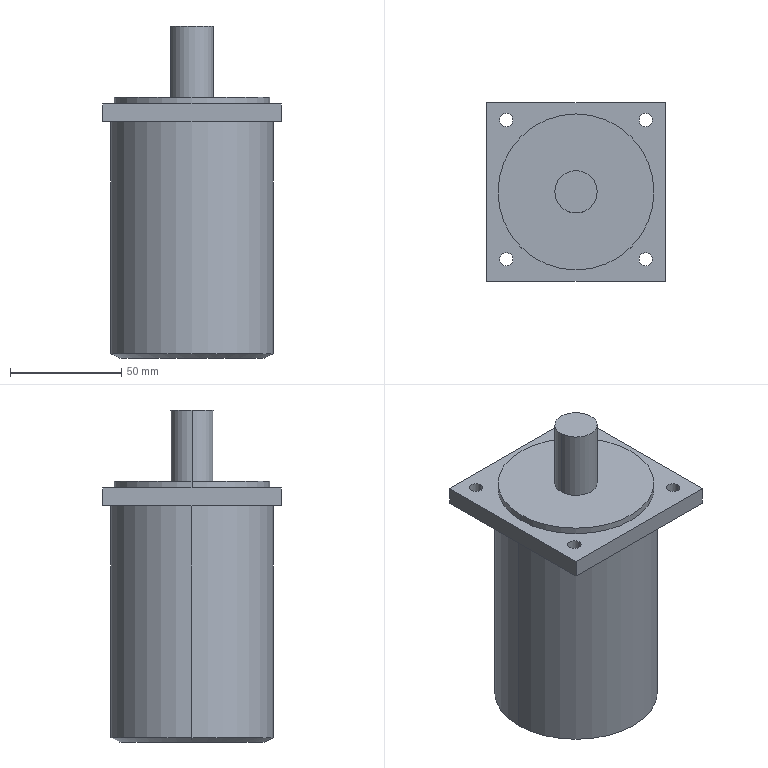Part | SolidWorks | features Boss 3, Chamfer 1, Cut 1, Extrusion 1 | 1 solid | 25 faces | box 80 x 80 x 149 mm | volume 513498 mm3 | cylinder 14 | plane 9 | cone 2 | commonest cylinder face diameters 6 x8 19 x2 70 x2 72.985 x2
STEP:
#1=CARTESIAN_POINT('',(7.508,40.,-106.));
#2=VERTEX_POINT('',#1);
#3=CARTESIAN_POINT('',(72.492,40.,-106.));
#4=VERTEX_POINT('',#3);
#5=CARTESIAN_POINT('',(40.,40.,-106.));
#6=DIRECTION('',(0.,0.,-1.));
#7=DIRECTION('',(-1.,0.,0.));
#8=AXIS2_PLACEMENT_3D('',#5,#6,#7);
#9=CIRCLE('',#8,32.492);
#10=EDGE_CURVE('',#2,#4,#9,.T.);
#11=ORIENTED_EDGE('',*,*,#10,.F.);
#12=CARTESIAN_POINT('',(3.508,40.,-104.));
#13=VERTEX_POINT('',#12);
#14=CARTESIAN_POINT('',(7.508,40.,-106.));
#15=DIRECTION('',(-0.8944,0.,0.4472));
#16=VECTOR('',#15,1000.);
#17=LINE('',#14,#16);
#18=EDGE_CURVE('',#2,#13,#17,.T.);
#19=ORIENTED_EDGE('',*,*,#18,.T.);
#20=CARTESIAN_POINT('',(76.492,40.,-104.));
#21=VERTEX_POINT('',#20);
#22=CARTESIAN_POINT('',(40.,40.,-104.));
#23=DIRECTION('',(0.,0.,1.));
#24=DIRECTION('',(-1.,0.,0.));
#25=AXIS2_PLACEMENT_3D('',#22,#23,#24);
#26=CIRCLE('',#25,36.492);
#27=EDGE_CURVE('',#21,#13,#26,.T.);
#28=ORIENTED_EDGE('',*,*,#27,.F.);
#29=CARTESIAN_POINT('',(72.492,40.,-106.));
#30=DIRECTION('',(0.8944,0.,0.4472));
#31=VECTOR('',#30,1000.);
#32=LINE('',#29,#31);
#33=EDGE_CURVE('',#4,#21,#32,.T.);
#34=ORIENTED_EDGE('',*,*,#33,.F.);
#35=EDGE_LOOP('',(#11,#19,#28,#34));
#36=FACE_OUTER_BOUND('',#35,.T.);
#37=CARTESIAN_POINT('',(40.,40.,-106.));
#38=DIRECTION('',(0.,0.,1.));
#39=DIRECTION('',(1.,0.,0.));
#40=AXIS2_PLACEMENT_3D('',#37,#38,#39);
#41=CONICAL_SURFACE('',#40,32.492,1.107);
#42=ADVANCED_FACE('',(#36),#41,.T.);
#43=CARTESIAN_POINT('',(5.714,9.772,0.));
#44=VERTEX_POINT('',#43);
#45=CARTESIAN_POINT('',(11.714,9.772,0.));
#46=VERTEX_POINT('',#45);
#47=CARTESIAN_POINT('',(8.714,9.772,0.));
#48=DIRECTION('',(0.,0.,1.));
#49=DIRECTION('',(-1.,0.,0.));
#50=AXIS2_PLACEMENT_3D('',#47,#48,#49);
#51=CIRCLE('',#50,3.);
#52=EDGE_CURVE('',#44,#46,#51,.T.);
#53=ORIENTED_EDGE('',*,*,#52,.F.);
#54=CARTESIAN_POINT('',(5.714,9.772,8.));
#55=VERTEX_POINT('',#54);
#56=CARTESIAN_POINT('',(5.714,9.772,-106.001));
#57=DIRECTION('',(0.,0.,1.));
#58=VECTOR('',#57,1000.);
#59=LINE('',#56,#58);
#60=EDGE_CURVE('',#44,#55,#59,.T.);
#61=ORIENTED_EDGE('',*,*,#60,.T.);
#62=CARTESIAN_POINT('',(11.714,9.772,8.));
#63=VERTEX_POINT('',#62);
#64=CARTESIAN_POINT('',(8.714,9.772,8.));
#65=DIRECTION('',(0.,0.,1.));
#66=DIRECTION('',(1.,0.,0.));
#67=AXIS2_PLACEMENT_3D('',#64,#65,#66);
#68=CIRCLE('',#67,3.);
#69=EDGE_CURVE('',#55,#63,#68,.T.);
#70=ORIENTED_EDGE('',*,*,#69,.T.);
#71=CARTESIAN_POINT('',(11.714,9.772,-106.001));
#72=DIRECTION('',(0.,0.,1.));
#73=VECTOR('',#72,1000.);
#74=LINE('',#71,#73);
#75=EDGE_CURVE('',#46,#63,#74,.T.);
#76=ORIENTED_EDGE('',*,*,#75,.F.);
#77=EDGE_LOOP('',(#53,#61,#70,#76));
#78=FACE_OUTER_BOUND('',#77,.T.);
#79=CARTESIAN_POINT('',(8.714,9.772,-106.001));
#80=DIRECTION('',(0.,0.,1.));
#81=DIRECTION('',(1.,0.,0.));
#82=AXIS2_PLACEMENT_3D('',#79,#80,#81);
#83=CYLINDRICAL_SURFACE('',#82,3.);
#84=ADVANCED_FACE('',(#78),#83,.F.);
#85=CARTESIAN_POINT('',(68.286,9.772,0.));
#86=VERTEX_POINT('',#85);
#87=CARTESIAN_POINT('',(74.286,9.772,0.));
#88=VERTEX_POINT('',#87);
#89=CARTESIAN_POINT('',(71.286,9.772,0.));
#90=DIRECTION('',(0.,0.,1.));
#91=DIRECTION('',(-1.,0.,0.));
#92=AXIS2_PLACEMENT_3D('',#89,#90,#91);
#93=CIRCLE('',#92,3.);
#94=EDGE_CURVE('',#86,#88,#93,.T.);
#95=ORIENTED_EDGE('',*,*,#94,.F.);
#96=CARTESIAN_POINT('',(68.286,9.772,8.));
#97=VERTEX_POINT('',#96);
#98=CARTESIAN_POINT('',(68.286,9.772,-106.001));
#99=DIRECTION('',(0.,0.,1.));
#100=VECTOR('',#99,1000.);
#101=LINE('',#98,#100);
#102=EDGE_CURVE('',#86,#97,#101,.T.);
#103=ORIENTED_EDGE('',*,*,#102,.T.);
#104=CARTESIAN_POINT('',(74.286,9.772,8.));
#105=VERTEX_POINT('',#104);
#106=CARTESIAN_POINT('',(71.286,9.772,8.));
#107=DIRECTION('',(0.,0.,1.));
#108=DIRECTION('',(1.,0.,0.));
#109=AXIS2_PLACEMENT_3D('',#106,#107,#108);
#110=CIRCLE('',#109,3.);
#111=EDGE_CURVE('',#97,#105,#110,.T.);
#112=ORIENTED_EDGE('',*,*,#111,.T.);
#113=CARTESIAN_POINT('',(74.286,9.772,-106.001));
#114=DIRECTION('',(0.,0.,1.));
#115=VECTOR('',#114,1000.);
#116=LINE('',#113,#115);
#117=EDGE_CURVE('',#88,#105,#116,.T.);
#118=ORIENTED_EDGE('',*,*,#117,.F.);
#119=EDGE_LOOP('',(#95,#103,#112,#118));
#120=FACE_OUTER_BOUND('',#119,.T.);
#121=CARTESIAN_POINT('',(71.286,9.772,-106.001));
#122=DIRECTION('',(0.,0.,1.));
#123=DIRECTION('',(1.,0.,0.));
#124=AXIS2_PLACEMENT_3D('',#121,#122,#123);
#125=CYLINDRICAL_SURFACE('',#124,3.);
#126=ADVANCED_FACE('',(#120),#125,.F.);
#127=CARTESIAN_POINT('',(68.286,72.344,0.));
#128=VERTEX_POINT('',#127);
#129=CARTESIAN_POINT('',(74.286,72.344,0.));
#130=VERTEX_POINT('',#129);
#131=CARTESIAN_POINT('',(71.286,72.344,0.));
#132=DIRECTION('',(0.,0.,1.));
#133=DIRECTION('',(-1.,0.,0.));
#134=AXIS2_PLACEMENT_3D('',#131,#132,#133);
#135=CIRCLE('',#134,3.);
#136=EDGE_CURVE('',#128,#130,#135,.T.);
#137=ORIENTED_EDGE('',*,*,#136,.F.);
#138=CARTESIAN_POINT('',(68.286,72.344,8.));
#139=VERTEX_POINT('',#138);
#140=CARTESIAN_POINT('',(68.286,72.344,-106.001));
#141=DIRECTION('',(0.,0.,1.));
#142=VECTOR('',#141,1000.);
#143=LINE('',#140,#142);
#144=EDGE_CURVE('',#128,#139,#143,.T.);
#145=ORIENTED_EDGE('',*,*,#144,.T.);
#146=CARTESIAN_POINT('',(74.286,72.344,8.));
#147=VERTEX_POINT('',#146);
#148=CARTESIAN_POINT('',(71.286,72.344,8.));
#149=DIRECTION('',(0.,0.,1.));
#150=DIRECTION('',(1.,0.,0.));
#151=AXIS2_PLACEMENT_3D('',#148,#149,#150);
#152=CIRCLE('',#151,3.);
#153=EDGE_CURVE('',#139,#147,#152,.T.);
#154=ORIENTED_EDGE('',*,*,#153,.T.);
#155=CARTESIAN_POINT('',(74.286,72.344,-106.001));
#156=DIRECTION('',(0.,0.,1.));
#157=VECTOR('',#156,1000.);
#158=LINE('',#155,#157);
#159=EDGE_CURVE('',#130,#147,#158,.T.);
#160=ORIENTED_EDGE('',*,*,#159,.F.);
#161=EDGE_LOOP('',(#137,#145,#154,#160));
#162=FACE_OUTER_BOUND('',#161,.T.);
#163=CARTESIAN_POINT('',(71.286,72.344,-106.001));
#164=DIRECTION('',(0.,0.,1.));
#165=DIRECTION('',(1.,0.,0.));
#166=AXIS2_PLACEMENT_3D('',#163,#164,#165);
#167=CYLINDRICAL_SURFACE('',#166,3.);
#168=ADVANCED_FACE('',(#162),#167,.F.);
#169=CARTESIAN_POINT('',(5.714,72.344,0.));
#170=VERTEX_POINT('',#169);
#171=CARTESIAN_POINT('',(11.714,72.344,0.));
#172=VERTEX_POINT('',#171);
#173=CARTESIAN_POINT('',(8.714,72.344,0.));
#174=DIRECTION('',(0.,0.,1.));
#175=DIRECTION('',(-1.,0.,0.));
#176=AXIS2_PLACEMENT_3D('',#173,#174,#175);
#177=CIRCLE('',#176,3.);
#178=EDGE_CURVE('',#170,#172,#177,.T.);
#179=ORIENTED_EDGE('',*,*,#178,.F.);
#180=CARTESIAN_POINT('',(5.714,72.344,8.));
#181=VERTEX_POINT('',#180);
#182=CARTESIAN_POINT('',(5.714,72.344,-106.001));
#183=DIRECTION('',(0.,0.,1.));
#184=VECTOR('',#183,1000.);
#185=LINE('',#182,#184);
#186=EDGE_CURVE('',#170,#181,#185,.T.);
#187=ORIENTED_EDGE('',*,*,#186,.T.);
#188=CARTESIAN_POINT('',(11.714,72.344,8.));
#189=VERTEX_POINT('',#188);
#190=CARTESIAN_POINT('',(8.714,72.344,8.));
#191=DIRECTION('',(0.,0.,1.));
#192=DIRECTION('',(1.,0.,0.));
#193=AXIS2_PLACEMENT_3D('',#190,#191,#192);
#194=CIRCLE('',#193,3.);
#195=EDGE_CURVE('',#181,#189,#194,.T.);
#196=ORIENTED_EDGE('',*,*,#195,.T.);
#197=CARTESIAN_POINT('',(11.714,72.344,-106.001));
#198=DIRECTION('',(0.,0.,1.));
#199=VECTOR('',#198,1000.);
#200=LINE('',#197,#199);
#201=EDGE_CURVE('',#172,#189,#200,.T.);
#202=ORIENTED_EDGE('',*,*,#201,.F.);
#203=EDGE_LOOP('',(#179,#187,#196,#202));
#204=FACE_OUTER_BOUND('',#203,.T.);
#205=CARTESIAN_POINT('',(8.714,72.344,-106.001));
#206=DIRECTION('',(0.,0.,1.));
#207=DIRECTION('',(1.,0.,0.));
#208=AXIS2_PLACEMENT_3D('',#205,#206,#207);
#209=CYLINDRICAL_SURFACE('',#208,3.);
#210=ADVANCED_FACE('',(#204),#209,.F.);
#211=ORIENTED_EDGE('',*,*,#27,.T.);
#212=CARTESIAN_POINT('',(3.508,40.,0.));
#213=VERTEX_POINT('',#212);
#214=CARTESIAN_POINT('',(3.508,40.,-106.));
#215=DIRECTION('',(0.,0.,1.));
#216=VECTOR('',#215,1000.);
#217=LINE('',#214,#216);
#218=EDGE_CURVE('',#13,#213,#217,.T.);
#219=ORIENTED_EDGE('',*,*,#218,.T.);
#220=CARTESIAN_POINT('',(76.492,40.,0.));
#221=VERTEX_POINT('',#220);
#222=CARTESIAN_POINT('',(40.,40.,0.));
#223=DIRECTION('',(0.,0.,-1.));
#224=DIRECTION('',(-1.,0.,0.));
#225=AXIS2_PLACEMENT_3D('',#222,#223,#224);
#226=CIRCLE('',#225,36.492);
#227=EDGE_CURVE('',#213,#221,#226,.T.);
#228=ORIENTED_EDGE('',*,*,#227,.T.);
#229=CARTESIAN_POINT('',(76.492,40.,-106.));
#230=DIRECTION('',(0.,0.,1.));
#231=VECTOR('',#230,1000.);
#232=LINE('',#229,#231);
#233=EDGE_CURVE('',#21,#221,#232,.T.);
#234=ORIENTED_EDGE('',*,*,#233,.F.);
#235=EDGE_LOOP('',(#211,#219,#228,#234));
#236=FACE_OUTER_BOUND('',#235,.T.);
#237=CARTESIAN_POINT('',(40.,40.,-106.));
#238=DIRECTION('',(0.,0.,1.));
#239=DIRECTION('',(1.,0.,0.));
#240=AXIS2_PLACEMENT_3D('',#237,#238,#239);
#241=CYLINDRICAL_SURFACE('',#240,36.492);
#242=ADVANCED_FACE('',(#236),#241,.T.);
#243=CARTESIAN_POINT('',(49.5,40.,43.));
#244=VERTEX_POINT('',#243);
#245=CARTESIAN_POINT('',(30.5,40.,43.));
#246=VERTEX_POINT('',#245);
#247=CARTESIAN_POINT('',(40.,40.,43.));
#248=DIRECTION('',(0.,0.,1.));
#249=DIRECTION('',(1.,0.,0.));
#250=AXIS2_PLACEMENT_3D('',#247,#248,#249);
#251=CIRCLE('',#250,9.5);
#252=EDGE_CURVE('',#244,#246,#251,.T.);
#253=ORIENTED_EDGE('',*,*,#252,.F.);
#254=CARTESIAN_POINT('',(49.5,40.,11.));
#255=VERTEX_POINT('',#254);
#256=CARTESIAN_POINT('',(49.5,40.,43.));
#257=DIRECTION('',(0.,0.,-1.));
#258=VECTOR('',#257,1000.);
#259=LINE('',#256,#258);
#260=EDGE_CURVE('',#244,#255,#259,.T.);
#261=ORIENTED_EDGE('',*,*,#260,.T.);
#262=CARTESIAN_POINT('',(30.5,40.,11.));
#263=VERTEX_POINT('',#262);
#264=CARTESIAN_POINT('',(40.,40.,11.));
#265=DIRECTION('',(0.,0.,1.));
#266=DIRECTION('',(1.,0.,0.));
#267=AXIS2_PLACEMENT_3D('',#264,#265,#266);
#268=CIRCLE('',#267,9.5);
#269=EDGE_CURVE('',#255,#263,#268,.T.);
#270=ORIENTED_EDGE('',*,*,#269,.T.);
#271=CARTESIAN_POINT('',(30.5,40.,43.));
#272=DIRECTION('',(0.,0.,-1.));
#273=VECTOR('',#272,1000.);
#274=LINE('',#271,#273);
#275=EDGE_CURVE('',#246,#263,#274,.T.);
#276=ORIENTED_EDGE('',*,*,#275,.F.);
#277=EDGE_LOOP('',(#253,#261,#270,#276));
#278=FACE_OUTER_BOUND('',#277,.T.);
#279=CARTESIAN_POINT('',(40.,40.,43.));
#280=DIRECTION('',(0.,0.,-1.));
#281=DIRECTION('',(-1.,0.,0.));
#282=AXIS2_PLACEMENT_3D('',#279,#280,#281);
#283=CYLINDRICAL_SURFACE('',#282,9.5);
#284=ADVANCED_FACE('',(#278),#283,.T.);
#285=CARTESIAN_POINT('',(75.,40.,11.));
#286=VERTEX_POINT('',#285);
#287=CARTESIAN_POINT('',(5.,40.,11.));
#288=VERTEX_POINT('',#287);
#289=CARTESIAN_POINT('',(40.,40.,11.));
#290=DIRECTION('',(0.,0.,1.));
#291=DIRECTION('',(1.,0.,0.));
#292=AXIS2_PLACEMENT_3D('',#289,#290,#291);
#293=CIRCLE('',#292,35.);
#294=EDGE_CURVE('',#286,#288,#293,.T.);
#295=ORIENTED_EDGE('',*,*,#294,.F.);
#296=CARTESIAN_POINT('',(75.,40.,8.));
#297=VERTEX_POINT('',#296);
#298=CARTESIAN_POINT('',(75.,40.,11.));
#299=DIRECTION('',(0.,0.,-1.));
#300=VECTOR('',#299,1000.);
#301=LINE('',#298,#300);
#302=EDGE_CURVE('',#286,#297,#301,.T.);
#303=ORIENTED_EDGE('',*,*,#302,.T.);
#304=CARTESIAN_POINT('',(5.,40.,8.));
#305=VERTEX_POINT('',#304);
#306=CARTESIAN_POINT('',(40.,40.,8.));
#307=DIRECTION('',(0.,0.,1.));
#308=DIRECTION('',(-1.,0.,0.));
#309=AXIS2_PLACEMENT_3D('',#306,#307,#308);
#310=CIRCLE('',#309,35.);
#311=EDGE_CURVE('',#297,#305,#310,.T.);
#312=ORIENTED_EDGE('',*,*,#311,.T.);
#313=CARTESIAN_POINT('',(5.,40.,11.));
#314=DIRECTION('',(0.,0.,-1.));
#315=VECTOR('',#314,1000.);
#316=LINE('',#313,#315);
#317=EDGE_CURVE('',#288,#305,#316,.T.);
#318=ORIENTED_EDGE('',*,*,#317,.F.);
#319=EDGE_LOOP('',(#295,#303,#312,#318));
#320=FACE_OUTER_BOUND('',#319,.T.);
#321=CARTESIAN_POINT('',(40.,40.,11.));
#322=DIRECTION('',(0.,0.,-1.));
#323=DIRECTION('',(-1.,0.,0.));
#324=AXIS2_PLACEMENT_3D('',#321,#322,#323);
#325=CYLINDRICAL_SURFACE('',#324,35.);
#326=ADVANCED_FACE('',(#320),#325,.T.);
#327=CARTESIAN_POINT('',(8.714,9.772,0.));
#328=DIRECTION('',(0.,0.,1.));
#329=DIRECTION('',(-1.,0.,0.));
#330=AXIS2_PLACEMENT_3D('',#327,#328,#329);
#331=CIRCLE('',#330,3.);
#332=EDGE_CURVE('',#46,#44,#331,.T.);
#333=ORIENTED_EDGE('',*,*,#332,.T.);
#334=ORIENTED_EDGE('',*,*,#52,.T.);
#335=EDGE_LOOP('',(#333,#334));
#336=FACE_BOUND('',#335,.T.);
#337=CARTESIAN_POINT('',(71.286,9.772,0.));
#338=DIRECTION('',(0.,0.,1.));
#339=DIRECTION('',(-1.,0.,0.));
#340=AXIS2_PLACEMENT_3D('',#337,#338,#339);
#341=CIRCLE('',#340,3.);
#342=EDGE_CURVE('',#88,#86,#341,.T.);
#343=ORIENTED_EDGE('',*,*,#342,.T.);
#344=ORIENTED_EDGE('',*,*,#94,.T.);
#345=EDGE_LOOP('',(#343,#344));
#346=FACE_BOUND('',#345,.T.);
#347=CARTESIAN_POINT('',(71.286,72.344,0.));
#348=DIRECTION('',(0.,0.,1.));
#349=DIRECTION('',(-1.,0.,0.));
#350=AXIS2_PLACEMENT_3D('',#347,#348,#349);
#351=CIRCLE('',#350,3.);
#352=EDGE_CURVE('',#130,#128,#351,.T.);
#353=ORIENTED_EDGE('',*,*,#352,.T.);
#354=ORIENTED_EDGE('',*,*,#136,.T.);
#355=EDGE_LOOP('',(#353,#354));
#356=FACE_BOUND('',#355,.T.);
#357=CARTESIAN_POINT('',(8.714,72.344,0.));
#358=DIRECTION('',(0.,0.,1.));
#359=DIRECTION('',(-1.,0.,0.));
#360=AXIS2_PLACEMENT_3D('',#357,#358,#359);
#361=CIRCLE('',#360,3.);
#362=EDGE_CURVE('',#172,#170,#361,.T.);
#363=ORIENTED_EDGE('',*,*,#362,.T.);
#364=ORIENTED_EDGE('',*,*,#178,.T.);
#365=EDGE_LOOP('',(#363,#364));
#366=FACE_BOUND('',#365,.T.);
#367=CARTESIAN_POINT('',(0.,80.,0.));
#368=VERTEX_POINT('',#367);
#369=CARTESIAN_POINT('',(0.,0.,0.));
#370=VERTEX_POINT('',#369);
#371=CARTESIAN_POINT('',(0.,0.,0.));
#372=DIRECTION('',(0.,-1.,0.));
#373=VECTOR('',#372,1000.);
#374=LINE('',#371,#373);
#375=EDGE_CURVE('',#368,#370,#374,.T.);
#376=ORIENTED_EDGE('',*,*,#375,.F.);
#377=CARTESIAN_POINT('',(80.,80.,0.));
#378=VERTEX_POINT('',#377);
#379=CARTESIAN_POINT('',(0.,80.,0.));
#380=DIRECTION('',(-1.,0.,0.));
#381=VECTOR('',#380,1000.);
#382=LINE('',#379,#381);
#383=EDGE_CURVE('',#378,#368,#382,.T.);
#384=ORIENTED_EDGE('',*,*,#383,.F.);
#385=CARTESIAN_POINT('',(80.,0.,0.));
#386=VERTEX_POINT('',#385);
#387=CARTESIAN_POINT('',(80.,0.,0.));
#388=DIRECTION('',(0.,1.,0.));
#389=VECTOR('',#388,1000.);
#390=LINE('',#387,#389);
#391=EDGE_CURVE('',#386,#378,#390,.T.);
#392=ORIENTED_EDGE('',*,*,#391,.F.);
#393=CARTESIAN_POINT('',(0.,0.,0.));
#394=DIRECTION('',(1.,0.,0.));
#395=VECTOR('',#394,1000.);
#396=LINE('',#393,#395);
#397=EDGE_CURVE('',#370,#386,#396,.T.);
#398=ORIENTED_EDGE('',*,*,#397,.F.);
#399=EDGE_LOOP('',(#376,#384,#392,#398));
#400=FACE_OUTER_BOUND('',#399,.T.);
#401=CARTESIAN_POINT('',(40.,40.,0.));
#402=DIRECTION('',(0.,0.,-1.));
#403=DIRECTION('',(-1.,0.,0.));
#404=AXIS2_PLACEMENT_3D('',#401,#402,#403);
#405=CIRCLE('',#404,36.492);
#406=EDGE_CURVE('',#221,#213,#405,.T.);
#407=ORIENTED_EDGE('',*,*,#406,.F.);
#408=ORIENTED_EDGE('',*,*,#227,.F.);
#409=EDGE_LOOP('',(#407,#408));
#410=FACE_BOUND('',#409,.T.);
#411=CARTESIAN_POINT('',(0.,80.,0.));
#412=DIRECTION('',(0.,0.,-1.));
#413=DIRECTION('',(-1.,0.,0.));
#414=AXIS2_PLACEMENT_3D('',#411,#412,#413);
#415=PLANE('',#414);
#416=ADVANCED_FACE('',(#336,#346,#356,#366,#400,#410),#415,.T.);
#417=CARTESIAN_POINT('',(40.,40.,11.));
#418=DIRECTION('',(0.,0.,1.));
#419=DIRECTION('',(1.,0.,0.));
#420=AXIS2_PLACEMENT_3D('',#417,#418,#419);
#421=CIRCLE('',#420,35.);
#422=EDGE_CURVE('',#288,#286,#421,.T.);
#423=ORIENTED_EDGE('',*,*,#422,.T.);
#424=ORIENTED_EDGE('',*,*,#294,.T.);
#425=EDGE_LOOP('',(#423,#424));
#426=FACE_OUTER_BOUND('',#425,.T.);
#427=CARTESIAN_POINT('',(40.,40.,11.));
#428=DIRECTION('',(0.,0.,1.));
#429=DIRECTION('',(1.,0.,0.));
#430=AXIS2_PLACEMENT_3D('',#427,#428,#429);
#431=CIRCLE('',#430,9.5);
#432=EDGE_CURVE('',#263,#255,#431,.T.);
#433=ORIENTED_EDGE('',*,*,#432,.F.);
#434=ORIENTED_EDGE('',*,*,#269,.F.);
#435=EDGE_LOOP('',(#433,#434));
#436=FACE_BOUND('',#435,.T.);
#437=CARTESIAN_POINT('',(40.,40.,11.));
#438=DIRECTION('',(0.,0.,1.));
#439=DIRECTION('',(1.,0.,0.));
#440=AXIS2_PLACEMENT_3D('',#437,#438,#439);
#441=PLANE('',#440);
#442=ADVANCED_FACE('',(#426,#436),#441,.T.);
#443=CARTESIAN_POINT('',(8.714,9.772,8.));
#444=DIRECTION('',(0.,0.,1.));
#445=DIRECTION('',(1.,0.,0.));
#446=AXIS2_PLACEMENT_3D('',#443,#444,#445);
#447=CIRCLE('',#446,3.);
#448=EDGE_CURVE('',#63,#55,#447,.T.);
#449=ORIENTED_EDGE('',*,*,#448,.F.);
#450=ORIENTED_EDGE('',*,*,#69,.F.);
#451=EDGE_LOOP('',(#449,#450));
#452=FACE_BOUND('',#451,.T.);
#453=CARTESIAN_POINT('',(71.286,9.772,8.));
#454=DIRECTION('',(0.,0.,1.));
#455=DIRECTION('',(1.,0.,0.));
#456=AXIS2_PLACEMENT_3D('',#453,#454,#455);
#457=CIRCLE('',#456,3.);
#458=EDGE_CURVE('',#105,#97,#457,.T.);
#459=ORIENTED_EDGE('',*,*,#458,.F.);
#460=ORIENTED_EDGE('',*,*,#111,.F.);
#461=EDGE_LOOP('',(#459,#460));
#462=FACE_BOUND('',#461,.T.);
#463=CARTESIAN_POINT('',(71.286,72.344,8.));
#464=DIRECTION('',(0.,0.,1.));
#465=DIRECTION('',(1.,0.,0.));
#466=AXIS2_PLACEMENT_3D('',#463,#464,#465);
#467=CIRCLE('',#466,3.);
#468=EDGE_CURVE('',#147,#139,#467,.T.);
#469=ORIENTED_EDGE('',*,*,#468,.F.);
#470=ORIENTED_EDGE('',*,*,#153,.F.);
#471=EDGE_LOOP('',(#469,#470));
#472=FACE_BOUND('',#471,.T.);
#473=CARTESIAN_POINT('',(8.714,72.344,8.));
#474=DIRECTION('',(0.,0.,1.));
#475=DIRECTION('',(1.,0.,0.));
#476=AXIS2_PLACEMENT_3D('',#473,#474,#475);
#477=CIRCLE('',#476,3.);
#478=EDGE_CURVE('',#189,#181,#477,.T.);
#479=ORIENTED_EDGE('',*,*,#478,.F.);
#480=ORIENTED_EDGE('',*,*,#195,.F.);
#481=EDGE_LOOP('',(#479,#480));
#482=FACE_BOUND('',#481,.T.);
#483=CARTESIAN_POINT('',(0.,80.,8.));
#484=VERTEX_POINT('',#483);
#485=CARTESIAN_POINT('',(0.,0.,8.));
#486=VERTEX_POINT('',#485);
#487=CARTESIAN_POINT('',(0.,0.,8.));
#488=DIRECTION('',(0.,-1.,0.));
#489=VECTOR('',#488,1000.);
#490=LINE('',#487,#489);
#491=EDGE_CURVE('',#484,#486,#490,.T.);
#492=ORIENTED_EDGE('',*,*,#491,.T.);
#493=CARTESIAN_POINT('',(80.,0.,8.));
#494=VERTEX_POINT('',#493);
#495=CARTESIAN_POINT('',(0.,0.,8.));
#496=DIRECTION('',(1.,0.,0.));
#497=VECTOR('',#496,1000.);
#498=LINE('',#495,#497);
#499=EDGE_CURVE('',#486,#494,#498,.T.);
#500=ORIENTED_EDGE('',*,*,#499,.T.);
#501=CARTESIAN_POINT('',(80.,80.,8.));
#502=VERTEX_POINT('',#501);
#503=CARTESIAN_POINT('',(80.,0.,8.));
#504=DIRECTION('',(0.,1.,0.));
#505=VECTOR('',#504,1000.);
#506=LINE('',#503,#505);
#507=EDGE_CURVE('',#494,#502,#506,.T.);
#508=ORIENTED_EDGE('',*,*,#507,.T.);
#509=CARTESIAN_POINT('',(0.,80.,8.));
#510=DIRECTION('',(-1.,0.,0.));
#511=VECTOR('',#510,1000.);
#512=LINE('',#509,#511);
#513=EDGE_CURVE('',#502,#484,#512,.T.);
#514=ORIENTED_EDGE('',*,*,#513,.T.);
#515=EDGE_LOOP('',(#492,#500,#508,#514));
#516=FACE_OUTER_BOUND('',#515,.T.);
#517=CARTESIAN_POINT('',(40.,40.,8.));
#518=DIRECTION('',(0.,0.,1.));
#519=DIRECTION('',(-1.,0.,0.));
#520=AXIS2_PLACEMENT_3D('',#517,#518,#519);
#521=CIRCLE('',#520,35.);
#522=EDGE_CURVE('',#305,#297,#521,.T.);
#523=ORIENTED_EDGE('',*,*,#522,.F.);
#524=ORIENTED_EDGE('',*,*,#311,.F.);
#525=EDGE_LOOP('',(#523,#524));
#526=FACE_BOUND('',#525,.T.);
#527=CARTESIAN_POINT('',(0.,80.,8.));
#528=DIRECTION('',(0.,0.,-1.));
#529=DIRECTION('',(-1.,0.,0.));
#530=AXIS2_PLACEMENT_3D('',#527,#528,#529);
#531=PLANE('',#530);
#532=ADVANCED_FACE('',(#452,#462,#472,#482,#516,#526),#531,.F.);
#533=ORIENTED_EDGE('',*,*,#375,.T.);
#534=CARTESIAN_POINT('',(0.,0.,8.));
#535=DIRECTION('',(0.,0.,-1.));
#536=VECTOR('',#535,1000.);
#537=LINE('',#534,#536);
#538=EDGE_CURVE('',#486,#370,#537,.T.);
#539=ORIENTED_EDGE('',*,*,#538,.F.);
#540=ORIENTED_EDGE('',*,*,#491,.F.);
#541=CARTESIAN_POINT('',(0.,80.,8.));
#542=DIRECTION('',(0.,0.,-1.));
#543=VECTOR('',#542,1000.);
#544=LINE('',#541,#543);
#545=EDGE_CURVE('',#484,#368,#544,.T.);
#546=ORIENTED_EDGE('',*,*,#545,.T.);
#547=EDGE_LOOP('',(#533,#539,#540,#546));
#548=FACE_OUTER_BOUND('',#547,.T.);
#549=CARTESIAN_POINT('',(0.,0.,8.));
#550=DIRECTION('',(1.,0.,0.));
#551=DIRECTION('',(0.,0.,-1.));
#552=AXIS2_PLACEMENT_3D('',#549,#550,#551);
#553=PLANE('',#552);
#554=ADVANCED_FACE('',(#548),#553,.F.);
#555=ORIENTED_EDGE('',*,*,#397,.T.);
#556=CARTESIAN_POINT('',(80.,0.,8.));
#557=DIRECTION('',(0.,0.,-1.));
#558=VECTOR('',#557,1000.);
#559=LINE('',#556,#558);
#560=EDGE_CURVE('',#494,#386,#559,.T.);
#561=ORIENTED_EDGE('',*,*,#560,.F.);
#562=ORIENTED_EDGE('',*,*,#499,.F.);
#563=ORIENTED_EDGE('',*,*,#538,.T.);
#564=EDGE_LOOP('',(#555,#561,#562,#563));
#565=FACE_OUTER_BOUND('',#564,.T.);
#566=CARTESIAN_POINT('',(0.,0.,8.));
#567=DIRECTION('',(0.,1.,0.));
#568=DIRECTION('',(0.,0.,1.));
#569=AXIS2_PLACEMENT_3D('',#566,#567,#568);
#570=PLANE('',#569);
#571=ADVANCED_FACE('',(#565),#570,.F.);
#572=ORIENTED_EDGE('',*,*,#391,.T.);
#573=CARTESIAN_POINT('',(80.,80.,8.));
#574=DIRECTION('',(0.,0.,-1.));
#575=VECTOR('',#574,1000.);
#576=LINE('',#573,#575);
#577=EDGE_CURVE('',#502,#378,#576,.T.);
#578=ORIENTED_EDGE('',*,*,#577,.F.);
#579=ORIENTED_EDGE('',*,*,#507,.F.);
#580=ORIENTED_EDGE('',*,*,#560,.T.);
#581=EDGE_LOOP('',(#572,#578,#579,#580));
#582=FACE_OUTER_BOUND('',#581,.T.);
#583=CARTESIAN_POINT('',(80.,0.,8.));
#584=DIRECTION('',(-1.,0.,0.));
#585=DIRECTION('',(0.,0.,1.));
#586=AXIS2_PLACEMENT_3D('',#583,#584,#585);
#587=PLANE('',#586);
#588=ADVANCED_FACE('',(#582),#587,.F.);
#589=ORIENTED_EDGE('',*,*,#383,.T.);
#590=ORIENTED_EDGE('',*,*,#545,.F.);
#591=ORIENTED_EDGE('',*,*,#513,.F.);
#592=ORIENTED_EDGE('',*,*,#577,.T.);
#593=EDGE_LOOP('',(#589,#590,#591,#592));
#594=FACE_OUTER_BOUND('',#593,.T.);
#595=CARTESIAN_POINT('',(0.,80.,8.));
#596=DIRECTION('',(0.,-1.,0.));
#597=DIRECTION('',(0.,0.,-1.));
#598=AXIS2_PLACEMENT_3D('',#595,#596,#597);
#599=PLANE('',#598);
#600=ADVANCED_FACE('',(#594),#599,.F.);
#601=ORIENTED_EDGE('',*,*,#302,.F.);
#602=ORIENTED_EDGE('',*,*,#422,.F.);
#603=ORIENTED_EDGE('',*,*,#317,.T.);
#604=ORIENTED_EDGE('',*,*,#522,.T.);
#605=EDGE_LOOP('',(#601,#602,#603,#604));
#606=FACE_OUTER_BOUND('',#605,.T.);
#607=CARTESIAN_POINT('',(40.,40.,11.));
#608=DIRECTION('',(0.,0.,-1.));
#609=DIRECTION('',(-1.,0.,0.));
#610=AXIS2_PLACEMENT_3D('',#607,#608,#609);
#611=CYLINDRICAL_SURFACE('',#610,35.);
#612=ADVANCED_FACE('',(#606),#611,.T.);
#613=ORIENTED_EDGE('',*,*,#260,.F.);
#614=CARTESIAN_POINT('',(40.,40.,43.));
#615=DIRECTION('',(0.,0.,1.));
#616=DIRECTION('',(1.,0.,0.));
#617=AXIS2_PLACEMENT_3D('',#614,#615,#616);
#618=CIRCLE('',#617,9.5);
#619=EDGE_CURVE('',#246,#244,#618,.T.);
#620=ORIENTED_EDGE('',*,*,#619,.F.);
#621=ORIENTED_EDGE('',*,*,#275,.T.);
#622=ORIENTED_EDGE('',*,*,#432,.T.);
#623=EDGE_LOOP('',(#613,#620,#621,#622));
#624=FACE_OUTER_BOUND('',#623,.T.);
#625=CARTESIAN_POINT('',(40.,40.,43.));
#626=DIRECTION('',(0.,0.,-1.));
#627=DIRECTION('',(-1.,0.,0.));
#628=AXIS2_PLACEMENT_3D('',#625,#626,#627);
#629=CYLINDRICAL_SURFACE('',#628,9.5);
#630=ADVANCED_FACE('',(#624),#629,.T.);
#631=ORIENTED_EDGE('',*,*,#619,.T.);
#632=ORIENTED_EDGE('',*,*,#252,.T.);
#633=EDGE_LOOP('',(#631,#632));
#634=FACE_OUTER_BOUND('',#633,.T.);
#635=CARTESIAN_POINT('',(40.,40.,43.));
#636=DIRECTION('',(0.,0.,1.));
#637=DIRECTION('',(1.,0.,0.));
#638=AXIS2_PLACEMENT_3D('',#635,#636,#637);
#639=PLANE('',#638);
#640=ADVANCED_FACE('',(#634),#639,.T.);
#641=ORIENTED_EDGE('',*,*,#218,.F.);
#642=CARTESIAN_POINT('',(40.,40.,-104.));
#643=DIRECTION('',(0.,0.,1.));
#644=DIRECTION('',(-1.,0.,0.));
#645=AXIS2_PLACEMENT_3D('',#642,#643,#644);
#646=CIRCLE('',#645,36.492);
#647=EDGE_CURVE('',#13,#21,#646,.T.);
#648=ORIENTED_EDGE('',*,*,#647,.T.);
#649=ORIENTED_EDGE('',*,*,#233,.T.);
#650=ORIENTED_EDGE('',*,*,#406,.T.);
#651=EDGE_LOOP('',(#641,#648,#649,#650));
#652=FACE_OUTER_BOUND('',#651,.T.);
#653=CARTESIAN_POINT('',(40.,40.,-106.));
#654=DIRECTION('',(0.,0.,1.));
#655=DIRECTION('',(1.,0.,0.));
#656=AXIS2_PLACEMENT_3D('',#653,#654,#655);
#657=CYLINDRICAL_SURFACE('',#656,36.492);
#658=ADVANCED_FACE('',(#652),#657,.T.);
#659=CARTESIAN_POINT('',(40.,40.,-106.));
#660=DIRECTION('',(0.,0.,-1.));
#661=DIRECTION('',(-1.,0.,0.));
#662=AXIS2_PLACEMENT_3D('',#659,#660,#661);
#663=CIRCLE('',#662,32.492);
#664=EDGE_CURVE('',#4,#2,#663,.T.);
#665=ORIENTED_EDGE('',*,*,#664,.T.);
#666=ORIENTED_EDGE('',*,*,#10,.T.);
#667=EDGE_LOOP('',(#665,#666));
#668=FACE_OUTER_BOUND('',#667,.T.);
#669=CARTESIAN_POINT('',(40.,40.,-106.));
#670=DIRECTION('',(0.,0.,-1.));
#671=DIRECTION('',(-1.,0.,0.));
#672=AXIS2_PLACEMENT_3D('',#669,#670,#671);
#673=PLANE('',#672);
#674=ADVANCED_FACE('',(#668),#673,.T.);
#675=ORIENTED_EDGE('',*,*,#186,.F.);
#676=ORIENTED_EDGE('',*,*,#362,.F.);
#677=ORIENTED_EDGE('',*,*,#201,.T.);
#678=ORIENTED_EDGE('',*,*,#478,.T.);
#679=EDGE_LOOP('',(#675,#676,#677,#678));
#680=FACE_OUTER_BOUND('',#679,.T.);
#681=CARTESIAN_POINT('',(8.714,72.344,-106.001));
#682=DIRECTION('',(0.,0.,1.));
#683=DIRECTION('',(1.,0.,0.));
#684=AXIS2_PLACEMENT_3D('',#681,#682,#683);
#685=CYLINDRICAL_SURFACE('',#684,3.);
#686=ADVANCED_FACE('',(#680),#685,.F.);
#687=ORIENTED_EDGE('',*,*,#144,.F.);
#688=ORIENTED_EDGE('',*,*,#352,.F.);
#689=ORIENTED_EDGE('',*,*,#159,.T.);
#690=ORIENTED_EDGE('',*,*,#468,.T.);
#691=EDGE_LOOP('',(#687,#688,#689,#690));
#692=FACE_OUTER_BOUND('',#691,.T.);
#693=CARTESIAN_POINT('',(71.286,72.344,-106.001));
#694=DIRECTION('',(0.,0.,1.));
#695=DIRECTION('',(1.,0.,0.));
#696=AXIS2_PLACEMENT_3D('',#693,#694,#695);
#697=CYLINDRICAL_SURFACE('',#696,3.);
#698=ADVANCED_FACE('',(#692),#697,.F.);
#699=ORIENTED_EDGE('',*,*,#102,.F.);
#700=ORIENTED_EDGE('',*,*,#342,.F.);
#701=ORIENTED_EDGE('',*,*,#117,.T.);
#702=ORIENTED_EDGE('',*,*,#458,.T.);
#703=EDGE_LOOP('',(#699,#700,#701,#702));
#704=FACE_OUTER_BOUND('',#703,.T.);
#705=CARTESIAN_POINT('',(71.286,9.772,-106.001));
#706=DIRECTION('',(0.,0.,1.));
#707=DIRECTION('',(1.,0.,0.));
#708=AXIS2_PLACEMENT_3D('',#705,#706,#707);
#709=CYLINDRICAL_SURFACE('',#708,3.);
#710=ADVANCED_FACE('',(#704),#709,.F.);
#711=ORIENTED_EDGE('',*,*,#60,.F.);
#712=ORIENTED_EDGE('',*,*,#332,.F.);
#713=ORIENTED_EDGE('',*,*,#75,.T.);
#714=ORIENTED_EDGE('',*,*,#448,.T.);
#715=EDGE_LOOP('',(#711,#712,#713,#714));
#716=FACE_OUTER_BOUND('',#715,.T.);
#717=CARTESIAN_POINT('',(8.714,9.772,-106.001));
#718=DIRECTION('',(0.,0.,1.));
#719=DIRECTION('',(1.,0.,0.));
#720=AXIS2_PLACEMENT_3D('',#717,#718,#719);
#721=CYLINDRICAL_SURFACE('',#720,3.);
#722=ADVANCED_FACE('',(#716),#721,.F.);
#723=ORIENTED_EDGE('',*,*,#18,.F.);
#724=ORIENTED_EDGE('',*,*,#664,.F.);
#725=ORIENTED_EDGE('',*,*,#33,.T.);
#726=ORIENTED_EDGE('',*,*,#647,.F.);
#727=EDGE_LOOP('',(#723,#724,#725,#726));
#728=FACE_OUTER_BOUND('',#727,.T.);
#729=CARTESIAN_POINT('',(40.,40.,-106.));
#730=DIRECTION('',(0.,0.,1.));
#731=DIRECTION('',(1.,0.,0.));
#732=AXIS2_PLACEMENT_3D('',#729,#730,#731);
#733=CONICAL_SURFACE('',#732,32.492,1.107);
#734=ADVANCED_FACE('',(#728),#733,.T.);
#735=CLOSED_SHELL('',(#42,#84,#126,#168,#210,#242,#284,#326,#416,#442,#532,#554,#571,#588,#600,#612,#630,#640,#658,#674,#686,#698,#710,#722,#734));
#736=MANIFOLD_SOLID_BREP('',#735);
#737=CARTESIAN_POINT('',(0.,0.,0.));
#738=DIRECTION('',(0.,0.,1.));
#739=DIRECTION('',(1.,0.,0.));
#740=AXIS2_PLACEMENT_3D('',#737,#738,#739);
#741=(LENGTH_UNIT()NAMED_UNIT(*)SI_UNIT(.MILLI.,.METRE.));
#742=UNCERTAINTY_MEASURE_WITH_UNIT(LENGTH_MEASURE(0.00001),#741,'','');
#743=(NAMED_UNIT(*)PLANE_ANGLE_UNIT()SI_UNIT($,.RADIAN.));
#744=(NAMED_UNIT(*)SI_UNIT($,.STERADIAN.)SOLID_ANGLE_UNIT());
#745=(GEOMETRIC_REPRESENTATION_CONTEXT(3)GLOBAL_UNCERTAINTY_ASSIGNED_CONTEXT((#742))GLOBAL_UNIT_ASSIGNED_CONTEXT((#741,#743,#744))REPRESENTATION_CONTEXT('',''));
#746=ADVANCED_BREP_SHAPE_REPRESENTATION('',(#736,#740),#745);